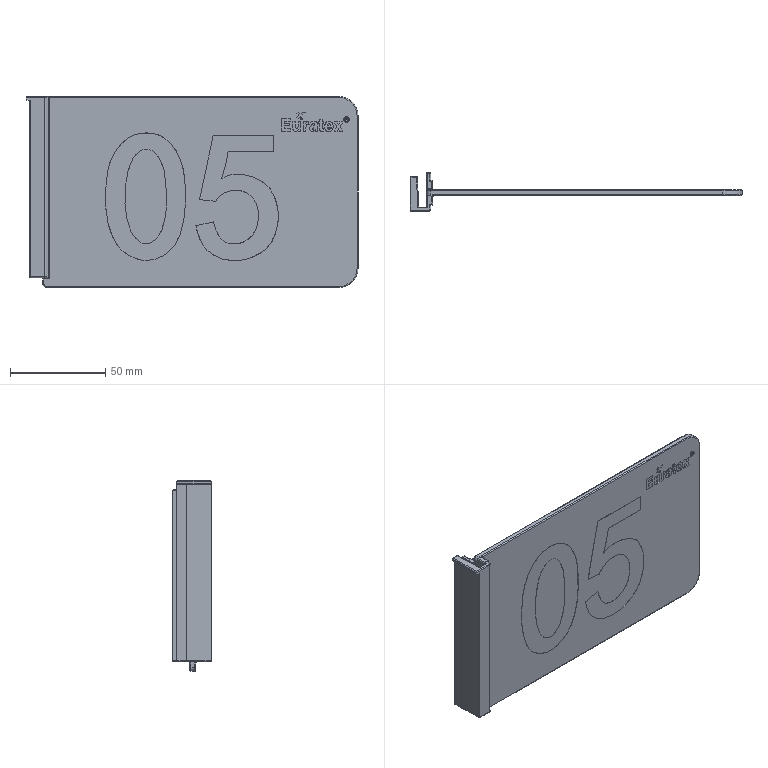Part | STEP file | 51E-01021SL10 | 1 solid | 379 faces | box 173.954 x 20.1 x 100 mm | volume 57536 mm3 | plane 238 | cylinder 75 | spline 50 | torus 16 | commonest cylinder face diameters 1 x46 0.448 x4 0.459 x4 0.83 x4 1.004 x4 2.422 x4